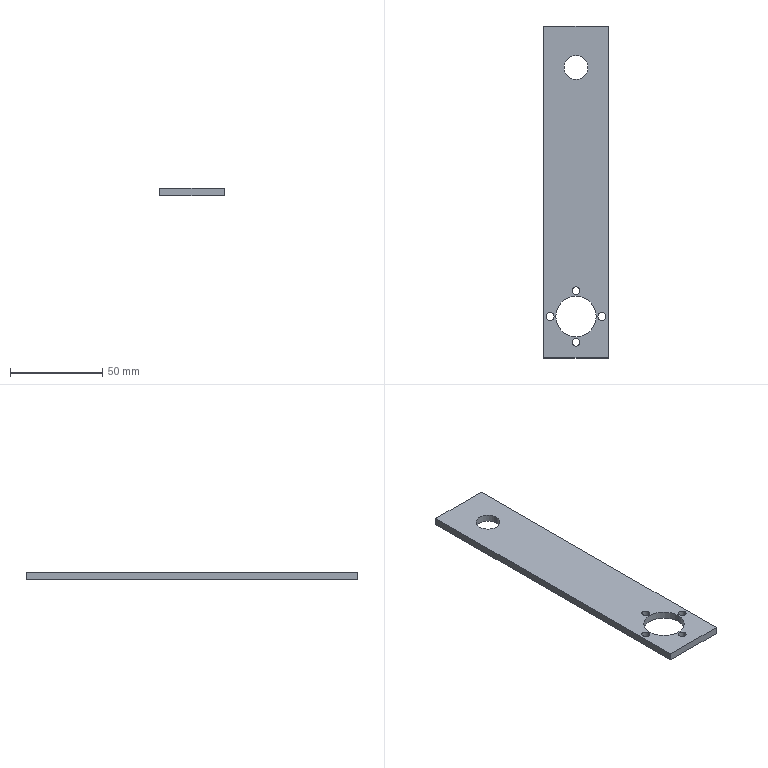Part | SolidWorks | features Extrusion 1, ICE 1 | 1 solid | 18 faces | box 35 x 180 x 4 mm | volume 22927 mm3 | cylinder 12 | plane 6 | commonest cylinder face diameters 4.2 x8 13 x2 22 x2
STEP:
#1=CARTESIAN_POINT('',(1.4,-157.5,0.));
#2=VERTEX_POINT('',#1);
#3=CARTESIAN_POINT('',(5.6,-157.5,0.));
#4=VERTEX_POINT('',#3);
#5=CARTESIAN_POINT('',(3.5,-157.5,0.));
#6=DIRECTION('',(0.,0.,1.));
#7=DIRECTION('',(1.,0.,0.));
#8=AXIS2_PLACEMENT_3D('',#5,#6,#7);
#9=CIRCLE('',#8,2.1);
#10=EDGE_CURVE('',#2,#4,#9,.T.);
#11=ORIENTED_EDGE('',*,*,#10,.F.);
#12=CARTESIAN_POINT('',(1.4,-157.5,4.));
#13=VERTEX_POINT('',#12);
#14=CARTESIAN_POINT('',(1.4,-157.5,-6.));
#15=DIRECTION('',(0.,0.,1.));
#16=VECTOR('',#15,1000.);
#17=LINE('',#14,#16);
#18=EDGE_CURVE('',#2,#13,#17,.T.);
#19=ORIENTED_EDGE('',*,*,#18,.T.);
#20=CARTESIAN_POINT('',(5.6,-157.5,4.));
#21=VERTEX_POINT('',#20);
#22=CARTESIAN_POINT('',(3.5,-157.5,4.));
#23=DIRECTION('',(0.,0.,1.));
#24=DIRECTION('',(1.,0.,0.));
#25=AXIS2_PLACEMENT_3D('',#22,#23,#24);
#26=CIRCLE('',#25,2.1);
#27=EDGE_CURVE('',#13,#21,#26,.T.);
#28=ORIENTED_EDGE('',*,*,#27,.T.);
#29=CARTESIAN_POINT('',(5.6,-157.5,-6.));
#30=DIRECTION('',(0.,0.,1.));
#31=VECTOR('',#30,1000.);
#32=LINE('',#29,#31);
#33=EDGE_CURVE('',#4,#21,#32,.T.);
#34=ORIENTED_EDGE('',*,*,#33,.F.);
#35=EDGE_LOOP('',(#11,#19,#28,#34));
#36=FACE_OUTER_BOUND('',#35,.T.);
#37=CARTESIAN_POINT('',(3.5,-157.5,-6.));
#38=DIRECTION('',(0.,0.,1.));
#39=DIRECTION('',(1.,0.,0.));
#40=AXIS2_PLACEMENT_3D('',#37,#38,#39);
#41=CYLINDRICAL_SURFACE('',#40,2.1);
#42=ADVANCED_FACE('',(#36),#41,.F.);
#43=CARTESIAN_POINT('',(15.4,-143.5,0.));
#44=VERTEX_POINT('',#43);
#45=CARTESIAN_POINT('',(19.6,-143.5,0.));
#46=VERTEX_POINT('',#45);
#47=CARTESIAN_POINT('',(17.5,-143.5,0.));
#48=DIRECTION('',(0.,0.,1.));
#49=DIRECTION('',(1.,0.,0.));
#50=AXIS2_PLACEMENT_3D('',#47,#48,#49);
#51=CIRCLE('',#50,2.1);
#52=EDGE_CURVE('',#44,#46,#51,.T.);
#53=ORIENTED_EDGE('',*,*,#52,.F.);
#54=CARTESIAN_POINT('',(15.4,-143.5,4.));
#55=VERTEX_POINT('',#54);
#56=CARTESIAN_POINT('',(15.4,-143.5,-6.));
#57=DIRECTION('',(0.,0.,1.));
#58=VECTOR('',#57,1000.);
#59=LINE('',#56,#58);
#60=EDGE_CURVE('',#44,#55,#59,.T.);
#61=ORIENTED_EDGE('',*,*,#60,.T.);
#62=CARTESIAN_POINT('',(19.6,-143.5,4.));
#63=VERTEX_POINT('',#62);
#64=CARTESIAN_POINT('',(17.5,-143.5,4.));
#65=DIRECTION('',(0.,0.,1.));
#66=DIRECTION('',(1.,0.,0.));
#67=AXIS2_PLACEMENT_3D('',#64,#65,#66);
#68=CIRCLE('',#67,2.1);
#69=EDGE_CURVE('',#55,#63,#68,.T.);
#70=ORIENTED_EDGE('',*,*,#69,.T.);
#71=CARTESIAN_POINT('',(19.6,-143.5,-6.));
#72=DIRECTION('',(0.,0.,1.));
#73=VECTOR('',#72,1000.);
#74=LINE('',#71,#73);
#75=EDGE_CURVE('',#46,#63,#74,.T.);
#76=ORIENTED_EDGE('',*,*,#75,.F.);
#77=EDGE_LOOP('',(#53,#61,#70,#76));
#78=FACE_OUTER_BOUND('',#77,.T.);
#79=CARTESIAN_POINT('',(17.5,-143.5,-6.));
#80=DIRECTION('',(0.,0.,1.));
#81=DIRECTION('',(1.,0.,0.));
#82=AXIS2_PLACEMENT_3D('',#79,#80,#81);
#83=CYLINDRICAL_SURFACE('',#82,2.1);
#84=ADVANCED_FACE('',(#78),#83,.F.);
#85=CARTESIAN_POINT('',(29.4,-157.5,0.));
#86=VERTEX_POINT('',#85);
#87=CARTESIAN_POINT('',(33.6,-157.5,0.));
#88=VERTEX_POINT('',#87);
#89=CARTESIAN_POINT('',(31.5,-157.5,0.));
#90=DIRECTION('',(0.,0.,1.));
#91=DIRECTION('',(1.,0.,0.));
#92=AXIS2_PLACEMENT_3D('',#89,#90,#91);
#93=CIRCLE('',#92,2.1);
#94=EDGE_CURVE('',#86,#88,#93,.T.);
#95=ORIENTED_EDGE('',*,*,#94,.F.);
#96=CARTESIAN_POINT('',(29.4,-157.5,4.));
#97=VERTEX_POINT('',#96);
#98=CARTESIAN_POINT('',(29.4,-157.5,-6.));
#99=DIRECTION('',(0.,0.,1.));
#100=VECTOR('',#99,1000.);
#101=LINE('',#98,#100);
#102=EDGE_CURVE('',#86,#97,#101,.T.);
#103=ORIENTED_EDGE('',*,*,#102,.T.);
#104=CARTESIAN_POINT('',(33.6,-157.5,4.));
#105=VERTEX_POINT('',#104);
#106=CARTESIAN_POINT('',(31.5,-157.5,4.));
#107=DIRECTION('',(0.,0.,1.));
#108=DIRECTION('',(1.,0.,0.));
#109=AXIS2_PLACEMENT_3D('',#106,#107,#108);
#110=CIRCLE('',#109,2.1);
#111=EDGE_CURVE('',#97,#105,#110,.T.);
#112=ORIENTED_EDGE('',*,*,#111,.T.);
#113=CARTESIAN_POINT('',(33.6,-157.5,-6.));
#114=DIRECTION('',(0.,0.,1.));
#115=VECTOR('',#114,1000.);
#116=LINE('',#113,#115);
#117=EDGE_CURVE('',#88,#105,#116,.T.);
#118=ORIENTED_EDGE('',*,*,#117,.F.);
#119=EDGE_LOOP('',(#95,#103,#112,#118));
#120=FACE_OUTER_BOUND('',#119,.T.);
#121=CARTESIAN_POINT('',(31.5,-157.5,-6.));
#122=DIRECTION('',(0.,0.,1.));
#123=DIRECTION('',(1.,0.,0.));
#124=AXIS2_PLACEMENT_3D('',#121,#122,#123);
#125=CYLINDRICAL_SURFACE('',#124,2.1);
#126=ADVANCED_FACE('',(#120),#125,.F.);
#127=CARTESIAN_POINT('',(15.4,-171.5,0.));
#128=VERTEX_POINT('',#127);
#129=CARTESIAN_POINT('',(19.6,-171.5,0.));
#130=VERTEX_POINT('',#129);
#131=CARTESIAN_POINT('',(17.5,-171.5,0.));
#132=DIRECTION('',(0.,0.,1.));
#133=DIRECTION('',(1.,0.,0.));
#134=AXIS2_PLACEMENT_3D('',#131,#132,#133);
#135=CIRCLE('',#134,2.1);
#136=EDGE_CURVE('',#128,#130,#135,.T.);
#137=ORIENTED_EDGE('',*,*,#136,.F.);
#138=CARTESIAN_POINT('',(15.4,-171.5,4.));
#139=VERTEX_POINT('',#138);
#140=CARTESIAN_POINT('',(15.4,-171.5,-6.));
#141=DIRECTION('',(0.,0.,1.));
#142=VECTOR('',#141,1000.);
#143=LINE('',#140,#142);
#144=EDGE_CURVE('',#128,#139,#143,.T.);
#145=ORIENTED_EDGE('',*,*,#144,.T.);
#146=CARTESIAN_POINT('',(19.6,-171.5,4.));
#147=VERTEX_POINT('',#146);
#148=CARTESIAN_POINT('',(17.5,-171.5,4.));
#149=DIRECTION('',(0.,0.,1.));
#150=DIRECTION('',(1.,0.,0.));
#151=AXIS2_PLACEMENT_3D('',#148,#149,#150);
#152=CIRCLE('',#151,2.1);
#153=EDGE_CURVE('',#139,#147,#152,.T.);
#154=ORIENTED_EDGE('',*,*,#153,.T.);
#155=CARTESIAN_POINT('',(19.6,-171.5,-6.));
#156=DIRECTION('',(0.,0.,1.));
#157=VECTOR('',#156,1000.);
#158=LINE('',#155,#157);
#159=EDGE_CURVE('',#130,#147,#158,.T.);
#160=ORIENTED_EDGE('',*,*,#159,.F.);
#161=EDGE_LOOP('',(#137,#145,#154,#160));
#162=FACE_OUTER_BOUND('',#161,.T.);
#163=CARTESIAN_POINT('',(17.5,-171.5,-6.));
#164=DIRECTION('',(0.,0.,1.));
#165=DIRECTION('',(1.,0.,0.));
#166=AXIS2_PLACEMENT_3D('',#163,#164,#165);
#167=CYLINDRICAL_SURFACE('',#166,2.1);
#168=ADVANCED_FACE('',(#162),#167,.F.);
#169=CARTESIAN_POINT('',(6.5,-157.5,4.));
#170=VERTEX_POINT('',#169);
#171=CARTESIAN_POINT('',(28.5,-157.5,4.));
#172=VERTEX_POINT('',#171);
#173=CARTESIAN_POINT('',(17.5,-157.5,4.));
#174=DIRECTION('',(0.,0.,1.));
#175=DIRECTION('',(1.,0.,0.));
#176=AXIS2_PLACEMENT_3D('',#173,#174,#175);
#177=CIRCLE('',#176,11.);
#178=EDGE_CURVE('',#170,#172,#177,.T.);
#179=ORIENTED_EDGE('',*,*,#178,.T.);
#180=CARTESIAN_POINT('',(28.5,-157.5,0.));
#181=VERTEX_POINT('',#180);
#182=CARTESIAN_POINT('',(28.5,-157.5,4.));
#183=DIRECTION('',(0.,0.,-1.));
#184=VECTOR('',#183,1000.);
#185=LINE('',#182,#184);
#186=EDGE_CURVE('',#172,#181,#185,.T.);
#187=ORIENTED_EDGE('',*,*,#186,.T.);
#188=CARTESIAN_POINT('',(6.5,-157.5,0.));
#189=VERTEX_POINT('',#188);
#190=CARTESIAN_POINT('',(17.5,-157.5,0.));
#191=DIRECTION('',(0.,0.,1.));
#192=DIRECTION('',(1.,0.,0.));
#193=AXIS2_PLACEMENT_3D('',#190,#191,#192);
#194=CIRCLE('',#193,11.);
#195=EDGE_CURVE('',#189,#181,#194,.T.);
#196=ORIENTED_EDGE('',*,*,#195,.F.);
#197=CARTESIAN_POINT('',(6.5,-157.5,4.));
#198=DIRECTION('',(0.,0.,-1.));
#199=VECTOR('',#198,1000.);
#200=LINE('',#197,#199);
#201=EDGE_CURVE('',#170,#189,#200,.T.);
#202=ORIENTED_EDGE('',*,*,#201,.F.);
#203=EDGE_LOOP('',(#179,#187,#196,#202));
#204=FACE_OUTER_BOUND('',#203,.T.);
#205=CARTESIAN_POINT('',(17.5,-157.5,4.));
#206=DIRECTION('',(0.,0.,-1.));
#207=DIRECTION('',(-1.,0.,0.));
#208=AXIS2_PLACEMENT_3D('',#205,#206,#207);
#209=CYLINDRICAL_SURFACE('',#208,11.);
#210=ADVANCED_FACE('',(#204),#209,.F.);
#211=CARTESIAN_POINT('',(11.,-22.5,4.));
#212=VERTEX_POINT('',#211);
#213=CARTESIAN_POINT('',(24.,-22.5,4.));
#214=VERTEX_POINT('',#213);
#215=CARTESIAN_POINT('',(17.5,-22.5,4.));
#216=DIRECTION('',(0.,0.,1.));
#217=DIRECTION('',(1.,0.,0.));
#218=AXIS2_PLACEMENT_3D('',#215,#216,#217);
#219=CIRCLE('',#218,6.5);
#220=EDGE_CURVE('',#212,#214,#219,.T.);
#221=ORIENTED_EDGE('',*,*,#220,.T.);
#222=CARTESIAN_POINT('',(24.,-22.5,0.));
#223=VERTEX_POINT('',#222);
#224=CARTESIAN_POINT('',(24.,-22.5,4.));
#225=DIRECTION('',(0.,0.,-1.));
#226=VECTOR('',#225,1000.);
#227=LINE('',#224,#226);
#228=EDGE_CURVE('',#214,#223,#227,.T.);
#229=ORIENTED_EDGE('',*,*,#228,.T.);
#230=CARTESIAN_POINT('',(11.,-22.5,0.));
#231=VERTEX_POINT('',#230);
#232=CARTESIAN_POINT('',(17.5,-22.5,0.));
#233=DIRECTION('',(0.,0.,1.));
#234=DIRECTION('',(1.,0.,0.));
#235=AXIS2_PLACEMENT_3D('',#232,#233,#234);
#236=CIRCLE('',#235,6.5);
#237=EDGE_CURVE('',#231,#223,#236,.T.);
#238=ORIENTED_EDGE('',*,*,#237,.F.);
#239=CARTESIAN_POINT('',(11.,-22.5,4.));
#240=DIRECTION('',(0.,0.,-1.));
#241=VECTOR('',#240,1000.);
#242=LINE('',#239,#241);
#243=EDGE_CURVE('',#212,#231,#242,.T.);
#244=ORIENTED_EDGE('',*,*,#243,.F.);
#245=EDGE_LOOP('',(#221,#229,#238,#244));
#246=FACE_OUTER_BOUND('',#245,.T.);
#247=CARTESIAN_POINT('',(17.5,-22.5,4.));
#248=DIRECTION('',(0.,0.,-1.));
#249=DIRECTION('',(-1.,0.,0.));
#250=AXIS2_PLACEMENT_3D('',#247,#248,#249);
#251=CYLINDRICAL_SURFACE('',#250,6.5);
#252=ADVANCED_FACE('',(#246),#251,.F.);
#253=CARTESIAN_POINT('',(3.5,-157.5,4.));
#254=DIRECTION('',(0.,0.,1.));
#255=DIRECTION('',(1.,0.,0.));
#256=AXIS2_PLACEMENT_3D('',#253,#254,#255);
#257=CIRCLE('',#256,2.1);
#258=EDGE_CURVE('',#21,#13,#257,.T.);
#259=ORIENTED_EDGE('',*,*,#258,.F.);
#260=ORIENTED_EDGE('',*,*,#27,.F.);
#261=EDGE_LOOP('',(#259,#260));
#262=FACE_BOUND('',#261,.T.);
#263=CARTESIAN_POINT('',(17.5,-143.5,4.));
#264=DIRECTION('',(0.,0.,1.));
#265=DIRECTION('',(1.,0.,0.));
#266=AXIS2_PLACEMENT_3D('',#263,#264,#265);
#267=CIRCLE('',#266,2.1);
#268=EDGE_CURVE('',#63,#55,#267,.T.);
#269=ORIENTED_EDGE('',*,*,#268,.F.);
#270=ORIENTED_EDGE('',*,*,#69,.F.);
#271=EDGE_LOOP('',(#269,#270));
#272=FACE_BOUND('',#271,.T.);
#273=CARTESIAN_POINT('',(31.5,-157.5,4.));
#274=DIRECTION('',(0.,0.,1.));
#275=DIRECTION('',(1.,0.,0.));
#276=AXIS2_PLACEMENT_3D('',#273,#274,#275);
#277=CIRCLE('',#276,2.1);
#278=EDGE_CURVE('',#105,#97,#277,.T.);
#279=ORIENTED_EDGE('',*,*,#278,.F.);
#280=ORIENTED_EDGE('',*,*,#111,.F.);
#281=EDGE_LOOP('',(#279,#280));
#282=FACE_BOUND('',#281,.T.);
#283=CARTESIAN_POINT('',(17.5,-171.5,4.));
#284=DIRECTION('',(0.,0.,1.));
#285=DIRECTION('',(1.,0.,0.));
#286=AXIS2_PLACEMENT_3D('',#283,#284,#285);
#287=CIRCLE('',#286,2.1);
#288=EDGE_CURVE('',#147,#139,#287,.T.);
#289=ORIENTED_EDGE('',*,*,#288,.F.);
#290=ORIENTED_EDGE('',*,*,#153,.F.);
#291=EDGE_LOOP('',(#289,#290));
#292=FACE_BOUND('',#291,.T.);
#293=ORIENTED_EDGE('',*,*,#220,.F.);
#294=CARTESIAN_POINT('',(17.5,-22.5,4.));
#295=DIRECTION('',(0.,0.,1.));
#296=DIRECTION('',(1.,0.,0.));
#297=AXIS2_PLACEMENT_3D('',#294,#295,#296);
#298=CIRCLE('',#297,6.5);
#299=EDGE_CURVE('',#214,#212,#298,.T.);
#300=ORIENTED_EDGE('',*,*,#299,.F.);
#301=EDGE_LOOP('',(#293,#300));
#302=FACE_BOUND('',#301,.T.);
#303=CARTESIAN_POINT('',(0.,0.,4.));
#304=VERTEX_POINT('',#303);
#305=CARTESIAN_POINT('',(0.,-180.,4.));
#306=VERTEX_POINT('',#305);
#307=CARTESIAN_POINT('',(0.,0.,4.));
#308=DIRECTION('',(0.,-1.,0.));
#309=VECTOR('',#308,1000.);
#310=LINE('',#307,#309);
#311=EDGE_CURVE('',#304,#306,#310,.T.);
#312=ORIENTED_EDGE('',*,*,#311,.T.);
#313=CARTESIAN_POINT('',(35.,-180.,4.));
#314=VERTEX_POINT('',#313);
#315=CARTESIAN_POINT('',(0.,-180.,4.));
#316=DIRECTION('',(1.,0.,0.));
#317=VECTOR('',#316,1000.);
#318=LINE('',#315,#317);
#319=EDGE_CURVE('',#306,#314,#318,.T.);
#320=ORIENTED_EDGE('',*,*,#319,.T.);
#321=CARTESIAN_POINT('',(35.,0.,4.));
#322=VERTEX_POINT('',#321);
#323=CARTESIAN_POINT('',(35.,0.,4.));
#324=DIRECTION('',(0.,1.,0.));
#325=VECTOR('',#324,1000.);
#326=LINE('',#323,#325);
#327=EDGE_CURVE('',#314,#322,#326,.T.);
#328=ORIENTED_EDGE('',*,*,#327,.T.);
#329=CARTESIAN_POINT('',(0.,0.,4.));
#330=DIRECTION('',(-1.,0.,0.));
#331=VECTOR('',#330,1000.);
#332=LINE('',#329,#331);
#333=EDGE_CURVE('',#322,#304,#332,.T.);
#334=ORIENTED_EDGE('',*,*,#333,.T.);
#335=EDGE_LOOP('',(#312,#320,#328,#334));
#336=FACE_OUTER_BOUND('',#335,.T.);
#337=ORIENTED_EDGE('',*,*,#178,.F.);
#338=CARTESIAN_POINT('',(17.5,-157.5,4.));
#339=DIRECTION('',(0.,0.,1.));
#340=DIRECTION('',(1.,0.,0.));
#341=AXIS2_PLACEMENT_3D('',#338,#339,#340);
#342=CIRCLE('',#341,11.);
#343=EDGE_CURVE('',#172,#170,#342,.T.);
#344=ORIENTED_EDGE('',*,*,#343,.F.);
#345=EDGE_LOOP('',(#337,#344));
#346=FACE_BOUND('',#345,.T.);
#347=CARTESIAN_POINT('',(0.,0.,4.));
#348=DIRECTION('',(0.,0.,1.));
#349=DIRECTION('',(1.,0.,0.));
#350=AXIS2_PLACEMENT_3D('',#347,#348,#349);
#351=PLANE('',#350);
#352=ADVANCED_FACE('',(#262,#272,#282,#292,#302,#336,#346),#351,.T.);
#353=CARTESIAN_POINT('',(3.5,-157.5,0.));
#354=DIRECTION('',(0.,0.,1.));
#355=DIRECTION('',(1.,0.,0.));
#356=AXIS2_PLACEMENT_3D('',#353,#354,#355);
#357=CIRCLE('',#356,2.1);
#358=EDGE_CURVE('',#4,#2,#357,.T.);
#359=ORIENTED_EDGE('',*,*,#358,.T.);
#360=ORIENTED_EDGE('',*,*,#10,.T.);
#361=EDGE_LOOP('',(#359,#360));
#362=FACE_BOUND('',#361,.T.);
#363=CARTESIAN_POINT('',(17.5,-143.5,0.));
#364=DIRECTION('',(0.,0.,1.));
#365=DIRECTION('',(1.,0.,0.));
#366=AXIS2_PLACEMENT_3D('',#363,#364,#365);
#367=CIRCLE('',#366,2.1);
#368=EDGE_CURVE('',#46,#44,#367,.T.);
#369=ORIENTED_EDGE('',*,*,#368,.T.);
#370=ORIENTED_EDGE('',*,*,#52,.T.);
#371=EDGE_LOOP('',(#369,#370));
#372=FACE_BOUND('',#371,.T.);
#373=CARTESIAN_POINT('',(31.5,-157.5,0.));
#374=DIRECTION('',(0.,0.,1.));
#375=DIRECTION('',(1.,0.,0.));
#376=AXIS2_PLACEMENT_3D('',#373,#374,#375);
#377=CIRCLE('',#376,2.1);
#378=EDGE_CURVE('',#88,#86,#377,.T.);
#379=ORIENTED_EDGE('',*,*,#378,.T.);
#380=ORIENTED_EDGE('',*,*,#94,.T.);
#381=EDGE_LOOP('',(#379,#380));
#382=FACE_BOUND('',#381,.T.);
#383=CARTESIAN_POINT('',(17.5,-171.5,0.));
#384=DIRECTION('',(0.,0.,1.));
#385=DIRECTION('',(1.,0.,0.));
#386=AXIS2_PLACEMENT_3D('',#383,#384,#385);
#387=CIRCLE('',#386,2.1);
#388=EDGE_CURVE('',#130,#128,#387,.T.);
#389=ORIENTED_EDGE('',*,*,#388,.T.);
#390=ORIENTED_EDGE('',*,*,#136,.T.);
#391=EDGE_LOOP('',(#389,#390));
#392=FACE_BOUND('',#391,.T.);
#393=CARTESIAN_POINT('',(0.,0.,0.));
#394=VERTEX_POINT('',#393);
#395=CARTESIAN_POINT('',(0.,-180.,0.));
#396=VERTEX_POINT('',#395);
#397=CARTESIAN_POINT('',(0.,0.,0.));
#398=DIRECTION('',(0.,-1.,0.));
#399=VECTOR('',#398,1000.);
#400=LINE('',#397,#399);
#401=EDGE_CURVE('',#394,#396,#400,.T.);
#402=ORIENTED_EDGE('',*,*,#401,.F.);
#403=CARTESIAN_POINT('',(35.,0.,0.));
#404=VERTEX_POINT('',#403);
#405=CARTESIAN_POINT('',(0.,0.,0.));
#406=DIRECTION('',(-1.,0.,0.));
#407=VECTOR('',#406,1000.);
#408=LINE('',#405,#407);
#409=EDGE_CURVE('',#404,#394,#408,.T.);
#410=ORIENTED_EDGE('',*,*,#409,.F.);
#411=CARTESIAN_POINT('',(35.,-180.,0.));
#412=VERTEX_POINT('',#411);
#413=CARTESIAN_POINT('',(35.,0.,0.));
#414=DIRECTION('',(0.,1.,0.));
#415=VECTOR('',#414,1000.);
#416=LINE('',#413,#415);
#417=EDGE_CURVE('',#412,#404,#416,.T.);
#418=ORIENTED_EDGE('',*,*,#417,.F.);
#419=CARTESIAN_POINT('',(0.,-180.,0.));
#420=DIRECTION('',(1.,0.,0.));
#421=VECTOR('',#420,1000.);
#422=LINE('',#419,#421);
#423=EDGE_CURVE('',#396,#412,#422,.T.);
#424=ORIENTED_EDGE('',*,*,#423,.F.);
#425=EDGE_LOOP('',(#402,#410,#418,#424));
#426=FACE_OUTER_BOUND('',#425,.T.);
#427=ORIENTED_EDGE('',*,*,#237,.T.);
#428=CARTESIAN_POINT('',(17.5,-22.5,0.));
#429=DIRECTION('',(0.,0.,1.));
#430=DIRECTION('',(1.,0.,0.));
#431=AXIS2_PLACEMENT_3D('',#428,#429,#430);
#432=CIRCLE('',#431,6.5);
#433=EDGE_CURVE('',#223,#231,#432,.T.);
#434=ORIENTED_EDGE('',*,*,#433,.T.);
#435=EDGE_LOOP('',(#427,#434));
#436=FACE_BOUND('',#435,.T.);
#437=ORIENTED_EDGE('',*,*,#195,.T.);
#438=CARTESIAN_POINT('',(17.5,-157.5,0.));
#439=DIRECTION('',(0.,0.,1.));
#440=DIRECTION('',(1.,0.,0.));
#441=AXIS2_PLACEMENT_3D('',#438,#439,#440);
#442=CIRCLE('',#441,11.);
#443=EDGE_CURVE('',#181,#189,#442,.T.);
#444=ORIENTED_EDGE('',*,*,#443,.T.);
#445=EDGE_LOOP('',(#437,#444));
#446=FACE_BOUND('',#445,.T.);
#447=CARTESIAN_POINT('',(0.,0.,0.));
#448=DIRECTION('',(0.,0.,1.));
#449=DIRECTION('',(1.,0.,0.));
#450=AXIS2_PLACEMENT_3D('',#447,#448,#449);
#451=PLANE('',#450);
#452=ADVANCED_FACE('',(#362,#372,#382,#392,#426,#436,#446),#451,.F.);
#453=ORIENTED_EDGE('',*,*,#401,.T.);
#454=CARTESIAN_POINT('',(0.,-180.,4.));
#455=DIRECTION('',(0.,0.,-1.));
#456=VECTOR('',#455,1000.);
#457=LINE('',#454,#456);
#458=EDGE_CURVE('',#306,#396,#457,.T.);
#459=ORIENTED_EDGE('',*,*,#458,.F.);
#460=ORIENTED_EDGE('',*,*,#311,.F.);
#461=CARTESIAN_POINT('',(0.,0.,4.));
#462=DIRECTION('',(0.,0.,-1.));
#463=VECTOR('',#462,1000.);
#464=LINE('',#461,#463);
#465=EDGE_CURVE('',#304,#394,#464,.T.);
#466=ORIENTED_EDGE('',*,*,#465,.T.);
#467=EDGE_LOOP('',(#453,#459,#460,#466));
#468=FACE_OUTER_BOUND('',#467,.T.);
#469=CARTESIAN_POINT('',(0.,0.,4.));
#470=DIRECTION('',(1.,0.,0.));
#471=DIRECTION('',(0.,1.,0.));
#472=AXIS2_PLACEMENT_3D('',#469,#470,#471);
#473=PLANE('',#472);
#474=ADVANCED_FACE('',(#468),#473,.F.);
#475=ORIENTED_EDGE('',*,*,#423,.T.);
#476=CARTESIAN_POINT('',(35.,-180.,4.));
#477=DIRECTION('',(0.,0.,-1.));
#478=VECTOR('',#477,1000.);
#479=LINE('',#476,#478);
#480=EDGE_CURVE('',#314,#412,#479,.T.);
#481=ORIENTED_EDGE('',*,*,#480,.F.);
#482=ORIENTED_EDGE('',*,*,#319,.F.);
#483=ORIENTED_EDGE('',*,*,#458,.T.);
#484=EDGE_LOOP('',(#475,#481,#482,#483));
#485=FACE_OUTER_BOUND('',#484,.T.);
#486=CARTESIAN_POINT('',(0.,-180.,4.));
#487=DIRECTION('',(0.,1.,0.));
#488=DIRECTION('',(0.,0.,1.));
#489=AXIS2_PLACEMENT_3D('',#486,#487,#488);
#490=PLANE('',#489);
#491=ADVANCED_FACE('',(#485),#490,.F.);
#492=ORIENTED_EDGE('',*,*,#417,.T.);
#493=CARTESIAN_POINT('',(35.,0.,4.));
#494=DIRECTION('',(0.,0.,-1.));
#495=VECTOR('',#494,1000.);
#496=LINE('',#493,#495);
#497=EDGE_CURVE('',#322,#404,#496,.T.);
#498=ORIENTED_EDGE('',*,*,#497,.F.);
#499=ORIENTED_EDGE('',*,*,#327,.F.);
#500=ORIENTED_EDGE('',*,*,#480,.T.);
#501=EDGE_LOOP('',(#492,#498,#499,#500));
#502=FACE_OUTER_BOUND('',#501,.T.);
#503=CARTESIAN_POINT('',(35.,0.,4.));
#504=DIRECTION('',(-1.,0.,0.));
#505=DIRECTION('',(0.,-1.,0.));
#506=AXIS2_PLACEMENT_3D('',#503,#504,#505);
#507=PLANE('',#506);
#508=ADVANCED_FACE('',(#502),#507,.F.);
#509=ORIENTED_EDGE('',*,*,#409,.T.);
#510=ORIENTED_EDGE('',*,*,#465,.F.);
#511=ORIENTED_EDGE('',*,*,#333,.F.);
#512=ORIENTED_EDGE('',*,*,#497,.T.);
#513=EDGE_LOOP('',(#509,#510,#511,#512));
#514=FACE_OUTER_BOUND('',#513,.T.);
#515=CARTESIAN_POINT('',(0.,0.,4.));
#516=DIRECTION('',(0.,-1.,0.));
#517=DIRECTION('',(0.,0.,-1.));
#518=AXIS2_PLACEMENT_3D('',#515,#516,#517);
#519=PLANE('',#518);
#520=ADVANCED_FACE('',(#514),#519,.F.);
#521=ORIENTED_EDGE('',*,*,#228,.F.);
#522=ORIENTED_EDGE('',*,*,#299,.T.);
#523=ORIENTED_EDGE('',*,*,#243,.T.);
#524=ORIENTED_EDGE('',*,*,#433,.F.);
#525=EDGE_LOOP('',(#521,#522,#523,#524));
#526=FACE_OUTER_BOUND('',#525,.T.);
#527=CARTESIAN_POINT('',(17.5,-22.5,4.));
#528=DIRECTION('',(0.,0.,-1.));
#529=DIRECTION('',(-1.,0.,0.));
#530=AXIS2_PLACEMENT_3D('',#527,#528,#529);
#531=CYLINDRICAL_SURFACE('',#530,6.5);
#532=ADVANCED_FACE('',(#526),#531,.F.);
#533=ORIENTED_EDGE('',*,*,#186,.F.);
#534=ORIENTED_EDGE('',*,*,#343,.T.);
#535=ORIENTED_EDGE('',*,*,#201,.T.);
#536=ORIENTED_EDGE('',*,*,#443,.F.);
#537=EDGE_LOOP('',(#533,#534,#535,#536));
#538=FACE_OUTER_BOUND('',#537,.T.);
#539=CARTESIAN_POINT('',(17.5,-157.5,4.));
#540=DIRECTION('',(0.,0.,-1.));
#541=DIRECTION('',(-1.,0.,0.));
#542=AXIS2_PLACEMENT_3D('',#539,#540,#541);
#543=CYLINDRICAL_SURFACE('',#542,11.);
#544=ADVANCED_FACE('',(#538),#543,.F.);
#545=ORIENTED_EDGE('',*,*,#144,.F.);
#546=ORIENTED_EDGE('',*,*,#388,.F.);
#547=ORIENTED_EDGE('',*,*,#159,.T.);
#548=ORIENTED_EDGE('',*,*,#288,.T.);
#549=EDGE_LOOP('',(#545,#546,#547,#548));
#550=FACE_OUTER_BOUND('',#549,.T.);
#551=CARTESIAN_POINT('',(17.5,-171.5,-6.));
#552=DIRECTION('',(0.,0.,1.));
#553=DIRECTION('',(1.,0.,0.));
#554=AXIS2_PLACEMENT_3D('',#551,#552,#553);
#555=CYLINDRICAL_SURFACE('',#554,2.1);
#556=ADVANCED_FACE('',(#550),#555,.F.);
#557=ORIENTED_EDGE('',*,*,#102,.F.);
#558=ORIENTED_EDGE('',*,*,#378,.F.);
#559=ORIENTED_EDGE('',*,*,#117,.T.);
#560=ORIENTED_EDGE('',*,*,#278,.T.);
#561=EDGE_LOOP('',(#557,#558,#559,#560));
#562=FACE_OUTER_BOUND('',#561,.T.);
#563=CARTESIAN_POINT('',(31.5,-157.5,-6.));
#564=DIRECTION('',(0.,0.,1.));
#565=DIRECTION('',(1.,0.,0.));
#566=AXIS2_PLACEMENT_3D('',#563,#564,#565);
#567=CYLINDRICAL_SURFACE('',#566,2.1);
#568=ADVANCED_FACE('',(#562),#567,.F.);
#569=ORIENTED_EDGE('',*,*,#60,.F.);
#570=ORIENTED_EDGE('',*,*,#368,.F.);
#571=ORIENTED_EDGE('',*,*,#75,.T.);
#572=ORIENTED_EDGE('',*,*,#268,.T.);
#573=EDGE_LOOP('',(#569,#570,#571,#572));
#574=FACE_OUTER_BOUND('',#573,.T.);
#575=CARTESIAN_POINT('',(17.5,-143.5,-6.));
#576=DIRECTION('',(0.,0.,1.));
#577=DIRECTION('',(1.,0.,0.));
#578=AXIS2_PLACEMENT_3D('',#575,#576,#577);
#579=CYLINDRICAL_SURFACE('',#578,2.1);
#580=ADVANCED_FACE('',(#574),#579,.F.);
#581=ORIENTED_EDGE('',*,*,#18,.F.);
#582=ORIENTED_EDGE('',*,*,#358,.F.);
#583=ORIENTED_EDGE('',*,*,#33,.T.);
#584=ORIENTED_EDGE('',*,*,#258,.T.);
#585=EDGE_LOOP('',(#581,#582,#583,#584));
#586=FACE_OUTER_BOUND('',#585,.T.);
#587=CARTESIAN_POINT('',(3.5,-157.5,-6.));
#588=DIRECTION('',(0.,0.,1.));
#589=DIRECTION('',(1.,0.,0.));
#590=AXIS2_PLACEMENT_3D('',#587,#588,#589);
#591=CYLINDRICAL_SURFACE('',#590,2.1);
#592=ADVANCED_FACE('',(#586),#591,.F.);
#593=CLOSED_SHELL('',(#42,#84,#126,#168,#210,#252,#352,#452,#474,#491,#508,#520,#532,#544,#556,#568,#580,#592));
#594=MANIFOLD_SOLID_BREP('',#593);
#595=CARTESIAN_POINT('',(0.,0.,0.));
#596=DIRECTION('',(0.,0.,1.));
#597=DIRECTION('',(1.,0.,0.));
#598=AXIS2_PLACEMENT_3D('',#595,#596,#597);
#599=(LENGTH_UNIT()NAMED_UNIT(*)SI_UNIT(.MILLI.,.METRE.));
#600=UNCERTAINTY_MEASURE_WITH_UNIT(LENGTH_MEASURE(0.00001),#599,'','');
#601=(NAMED_UNIT(*)PLANE_ANGLE_UNIT()SI_UNIT($,.RADIAN.));
#602=(NAMED_UNIT(*)SI_UNIT($,.STERADIAN.)SOLID_ANGLE_UNIT());
#603=(GEOMETRIC_REPRESENTATION_CONTEXT(3)GLOBAL_UNCERTAINTY_ASSIGNED_CONTEXT((#600))GLOBAL_UNIT_ASSIGNED_CONTEXT((#599,#601,#602))REPRESENTATION_CONTEXT('',''));
#604=ADVANCED_BREP_SHAPE_REPRESENTATION('',(#594,#598),#603);